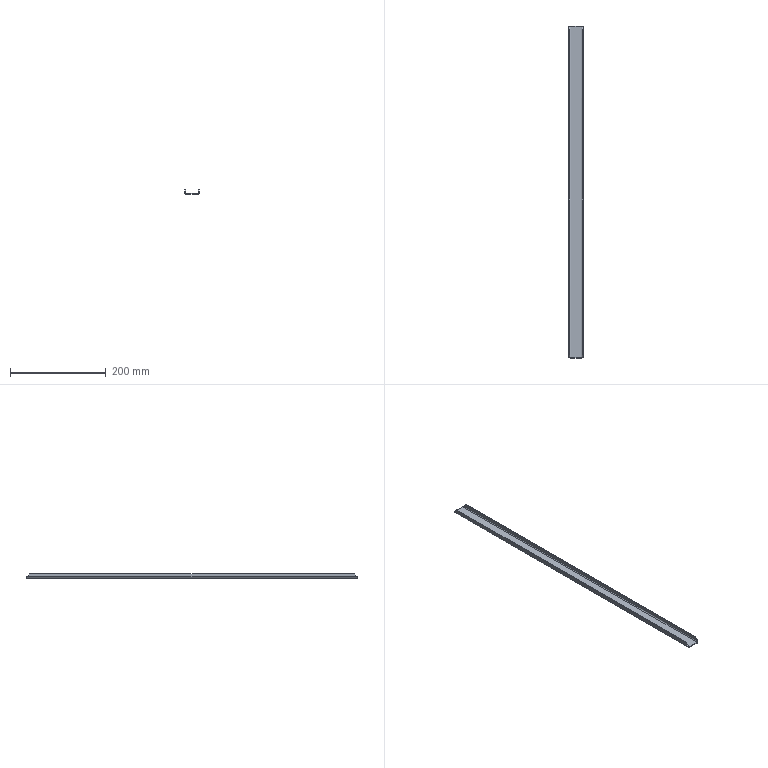Part | NX | features solid 2 | 1 solid | 22 faces | box 30 x 694.177 x 10 mm | volume 60022 mm3 | plane 14 | spline 4 | cylinder 4 | commonest cylinder face diameters 4 x2 8 x2
STEP:
#1=CARTESIAN_POINT('',(1379.,-1435.089,1444.8));
#2=VERTEX_POINT('',#1);
#3=CARTESIAN_POINT('',(1401.,-1435.089,1444.8));
#4=VERTEX_POINT('',#3);
#5=CARTESIAN_POINT('',(1405.,-1435.089,1444.8));
#6=DIRECTION('',(1.,0.,0.));
#7=VECTOR('',#6,1000.);
#8=LINE('',#5,#7);
#9=EDGE_CURVE('',#2,#4,#8,.T.);
#10=ORIENTED_EDGE('',*,*,#9,.T.);
#11=CARTESIAN_POINT('',(1401.,-1435.089,1446.8));
#12=VERTEX_POINT('',#11);
#13=CARTESIAN_POINT('',(1401.,-1435.089,1446.8));
#14=DIRECTION('',(0.,0.,1.));
#15=VECTOR('',#14,1000.);
#16=LINE('',#13,#15);
#17=EDGE_CURVE('',#4,#12,#16,.T.);
#18=ORIENTED_EDGE('',*,*,#17,.T.);
#19=CARTESIAN_POINT('',(1379.,-1435.089,1446.8));
#20=VERTEX_POINT('',#19);
#21=CARTESIAN_POINT('',(1405.,-1435.089,1446.8));
#22=DIRECTION('',(1.,0.,0.));
#23=VECTOR('',#22,1000.);
#24=LINE('',#21,#23);
#25=EDGE_CURVE('',#20,#12,#24,.T.);
#26=ORIENTED_EDGE('',*,*,#25,.F.);
#27=CARTESIAN_POINT('',(1379.,-1435.089,1446.8));
#28=DIRECTION('',(0.,0.,1.));
#29=VECTOR('',#28,1000.);
#30=LINE('',#27,#29);
#31=EDGE_CURVE('',#2,#20,#30,.T.);
#32=ORIENTED_EDGE('',*,*,#31,.F.);
#33=EDGE_LOOP('',(#10,#18,#26,#32));
#34=FACE_BOUND('',#33,.T.);
#35=CARTESIAN_POINT('',(1405.,-1435.089,1446.8));
#36=DIRECTION('',(0.,1.,0.));
#37=DIRECTION('',(0.,0.,-1.));
#38=AXIS2_PLACEMENT_3D('',#35,#36,#37);
#39=PLANE('',#38);
#40=ADVANCED_FACE('',(#34),#39,.F.);
#41=CARTESIAN_POINT('',(1403.,-1433.089,1448.8));
#42=VERTEX_POINT('',#41);
#43=CARTESIAN_POINT('',(1405.,-1433.089,1448.8));
#44=VERTEX_POINT('',#43);
#45=CARTESIAN_POINT('',(1405.,-1433.089,1448.8));
#46=DIRECTION('',(1.,0.,0.));
#47=VECTOR('',#46,1000.);
#48=LINE('',#45,#47);
#49=EDGE_CURVE('',#42,#44,#48,.T.);
#50=ORIENTED_EDGE('',*,*,#49,.F.);
#51=CARTESIAN_POINT('',(1401.,-1435.089,1446.8));
#52=CARTESIAN_POINT('',(1402.172,-1435.089,1446.8));
#53=CARTESIAN_POINT('',(1403.,-1434.26,1447.628));
#54=CARTESIAN_POINT('',(1403.,-1433.089,1448.8));
#55=(BOUNDED_CURVE()B_SPLINE_CURVE(3,(#51,#52,#53,#54),.UNSPECIFIED.,.F.,.F.)B_SPLINE_CURVE_WITH_KNOTS((4,4),(3.142,4.712),.PIECEWISE_BEZIER_KNOTS.)CURVE()GEOMETRIC_REPRESENTATION_ITEM()RATIONAL_B_SPLINE_CURVE((1.,0.8047,0.8047,1.))REPRESENTATION_ITEM(''));
#56=EDGE_CURVE('',#12,#42,#55,.T.);
#57=ORIENTED_EDGE('',*,*,#56,.F.);
#58=ORIENTED_EDGE('',*,*,#17,.F.);
#59=CARTESIAN_POINT('',(1401.,-1435.089,1444.8));
#60=CARTESIAN_POINT('',(1403.343,-1435.089,1444.8));
#61=CARTESIAN_POINT('',(1405.,-1434.26,1446.457));
#62=CARTESIAN_POINT('',(1405.,-1433.089,1448.8));
#63=(BOUNDED_CURVE()B_SPLINE_CURVE(3,(#59,#60,#61,#62),.UNSPECIFIED.,.F.,.F.)B_SPLINE_CURVE_WITH_KNOTS((4,4),(3.142,4.712),.PIECEWISE_BEZIER_KNOTS.)CURVE()GEOMETRIC_REPRESENTATION_ITEM()RATIONAL_B_SPLINE_CURVE((1.,0.8047,0.8047,1.))REPRESENTATION_ITEM(''));
#64=EDGE_CURVE('',#4,#44,#63,.T.);
#65=ORIENTED_EDGE('',*,*,#64,.T.);
#66=EDGE_LOOP('',(#50,#57,#58,#65));
#67=FACE_BOUND('',#66,.T.);
#68=CARTESIAN_POINT('',(1401.,-1435.089,1444.8));
#69=CARTESIAN_POINT('',(1401.,-1435.089,1445.467));
#70=CARTESIAN_POINT('',(1401.,-1435.089,1446.133));
#71=CARTESIAN_POINT('',(1401.,-1435.089,1446.8));
#72=CARTESIAN_POINT('',(1403.,-1435.089,1444.8));
#73=CARTESIAN_POINT('',(1402.667,-1435.089,1445.467));
#74=CARTESIAN_POINT('',(1402.333,-1435.089,1446.133));
#75=CARTESIAN_POINT('',(1402.,-1435.089,1446.8));
#76=CARTESIAN_POINT('',(1405.,-1434.422,1446.133));
#77=CARTESIAN_POINT('',(1404.333,-1434.422,1446.578));
#78=CARTESIAN_POINT('',(1403.667,-1434.422,1447.022));
#79=CARTESIAN_POINT('',(1403.,-1434.422,1447.467));
#80=CARTESIAN_POINT('',(1405.,-1433.089,1448.8));
#81=CARTESIAN_POINT('',(1404.333,-1433.089,1448.8));
#82=CARTESIAN_POINT('',(1403.667,-1433.089,1448.8));
#83=CARTESIAN_POINT('',(1403.,-1433.089,1448.8));
#84=(BOUNDED_SURFACE()B_SPLINE_SURFACE(3,3,((#68,#69,#70,#71),(#72,#73,#74,#75),(#76,#77,#78,#79),(#80,#81,#82,#83)),.UNSPECIFIED.,.F.,.F.,.F.)B_SPLINE_SURFACE_WITH_KNOTS((4,4),(4,4),(0.5,0.75),(0.,1.),.PIECEWISE_BEZIER_KNOTS.)GEOMETRIC_REPRESENTATION_ITEM()RATIONAL_B_SPLINE_SURFACE(((1.,1.,1.,1.),(0.6667,0.6667,0.6667,0.6667),(0.5,0.5,0.5,0.5),(0.5,0.5,0.5,0.5)))REPRESENTATION_ITEM('')SURFACE());
#85=ADVANCED_FACE('',(#67),#84,.T.);
#86=CARTESIAN_POINT('',(1375.,-1433.089,1448.8));
#87=VERTEX_POINT('',#86);
#88=CARTESIAN_POINT('',(1377.,-1433.089,1448.8));
#89=VERTEX_POINT('',#88);
#90=CARTESIAN_POINT('',(1377.,-1433.089,1448.8));
#91=DIRECTION('',(1.,0.,0.));
#92=VECTOR('',#91,1000.);
#93=LINE('',#90,#92);
#94=EDGE_CURVE('',#87,#89,#93,.T.);
#95=ORIENTED_EDGE('',*,*,#94,.T.);
#96=CARTESIAN_POINT('',(1377.,-1427.089,1454.8));
#97=VERTEX_POINT('',#96);
#98=CARTESIAN_POINT('',(1377.,-1436.294,1445.594));
#99=DIRECTION('',(0.,-0.7071,-0.7071));
#100=VECTOR('',#99,1000.);
#101=LINE('',#98,#100);
#102=EDGE_CURVE('',#97,#89,#101,.T.);
#103=ORIENTED_EDGE('',*,*,#102,.F.);
#104=CARTESIAN_POINT('',(1375.,-1427.089,1454.8));
#105=VERTEX_POINT('',#104);
#106=CARTESIAN_POINT('',(1377.,-1427.089,1454.8));
#107=DIRECTION('',(1.,0.,0.));
#108=VECTOR('',#107,1000.);
#109=LINE('',#106,#108);
#110=EDGE_CURVE('',#105,#97,#109,.T.);
#111=ORIENTED_EDGE('',*,*,#110,.F.);
#112=CARTESIAN_POINT('',(1375.,-1436.294,1445.594));
#113=DIRECTION('',(0.,-0.7071,-0.7071));
#114=VECTOR('',#113,1000.);
#115=LINE('',#112,#114);
#116=EDGE_CURVE('',#105,#87,#115,.T.);
#117=ORIENTED_EDGE('',*,*,#116,.T.);
#118=EDGE_LOOP('',(#95,#103,#111,#117));
#119=FACE_BOUND('',#118,.T.);
#120=CARTESIAN_POINT('',(1377.,-1436.294,1445.594));
#121=DIRECTION('',(0.,0.7071,-0.7071));
#122=DIRECTION('',(-1.,0.,0.));
#123=AXIS2_PLACEMENT_3D('',#120,#121,#122);
#124=PLANE('',#123);
#125=ADVANCED_FACE('',(#119),#124,.F.);
#126=ORIENTED_EDGE('',*,*,#31,.T.);
#127=CARTESIAN_POINT('',(1377.,-1433.089,1448.8));
#128=CARTESIAN_POINT('',(1377.,-1434.26,1447.628));
#129=CARTESIAN_POINT('',(1377.828,-1435.089,1446.8));
#130=CARTESIAN_POINT('',(1379.,-1435.089,1446.8));
#131=(BOUNDED_CURVE()B_SPLINE_CURVE(3,(#127,#128,#129,#130),.UNSPECIFIED.,.F.,.F.)B_SPLINE_CURVE_WITH_KNOTS((4,4),(1.571,3.142),.PIECEWISE_BEZIER_KNOTS.)CURVE()GEOMETRIC_REPRESENTATION_ITEM()RATIONAL_B_SPLINE_CURVE((1.,0.8047,0.8047,1.))REPRESENTATION_ITEM(''));
#132=EDGE_CURVE('',#89,#20,#131,.T.);
#133=ORIENTED_EDGE('',*,*,#132,.F.);
#134=ORIENTED_EDGE('',*,*,#94,.F.);
#135=CARTESIAN_POINT('',(1375.,-1433.089,1448.8));
#136=CARTESIAN_POINT('',(1375.,-1434.26,1446.457));
#137=CARTESIAN_POINT('',(1376.657,-1435.089,1444.8));
#138=CARTESIAN_POINT('',(1379.,-1435.089,1444.8));
#139=(BOUNDED_CURVE()B_SPLINE_CURVE(3,(#135,#136,#137,#138),.UNSPECIFIED.,.F.,.F.)B_SPLINE_CURVE_WITH_KNOTS((4,4),(1.571,3.142),.PIECEWISE_BEZIER_KNOTS.)CURVE()GEOMETRIC_REPRESENTATION_ITEM()RATIONAL_B_SPLINE_CURVE((1.,0.8047,0.8047,1.))REPRESENTATION_ITEM(''));
#140=EDGE_CURVE('',#87,#2,#139,.T.);
#141=ORIENTED_EDGE('',*,*,#140,.T.);
#142=EDGE_LOOP('',(#126,#133,#134,#141));
#143=FACE_BOUND('',#142,.T.);
#144=CARTESIAN_POINT('',(1375.,-1433.089,1448.8));
#145=CARTESIAN_POINT('',(1375.667,-1433.089,1448.8));
#146=CARTESIAN_POINT('',(1376.333,-1433.089,1448.8));
#147=CARTESIAN_POINT('',(1377.,-1433.089,1448.8));
#148=CARTESIAN_POINT('',(1375.,-1434.422,1446.133));
#149=CARTESIAN_POINT('',(1375.667,-1434.422,1446.578));
#150=CARTESIAN_POINT('',(1376.333,-1434.422,1447.022));
#151=CARTESIAN_POINT('',(1377.,-1434.422,1447.467));
#152=CARTESIAN_POINT('',(1377.,-1435.089,1444.8));
#153=CARTESIAN_POINT('',(1377.333,-1435.089,1445.467));
#154=CARTESIAN_POINT('',(1377.667,-1435.089,1446.133));
#155=CARTESIAN_POINT('',(1378.,-1435.089,1446.8));
#156=CARTESIAN_POINT('',(1379.,-1435.089,1444.8));
#157=CARTESIAN_POINT('',(1379.,-1435.089,1445.467));
#158=CARTESIAN_POINT('',(1379.,-1435.089,1446.133));
#159=CARTESIAN_POINT('',(1379.,-1435.089,1446.8));
#160=(BOUNDED_SURFACE()B_SPLINE_SURFACE(3,3,((#144,#145,#146,#147),(#148,#149,#150,#151),(#152,#153,#154,#155),(#156,#157,#158,#159)),.UNSPECIFIED.,.F.,.F.,.F.)B_SPLINE_SURFACE_WITH_KNOTS((4,4),(4,4),(0.25,0.5),(0.,1.),.PIECEWISE_BEZIER_KNOTS.)GEOMETRIC_REPRESENTATION_ITEM()RATIONAL_B_SPLINE_SURFACE(((0.5,0.5,0.5,0.5),(0.5,0.5,0.5,0.5),(0.6667,0.6667,0.6667,0.6667),(1.,1.,1.,1.)))REPRESENTATION_ITEM('')SURFACE());
#161=ADVANCED_FACE('',(#143),#160,.T.);
#162=ORIENTED_EDGE('',*,*,#49,.T.);
#163=CARTESIAN_POINT('',(1405.,-1427.089,1454.8));
#164=VERTEX_POINT('',#163);
#165=CARTESIAN_POINT('',(1405.,-1431.294,1450.594));
#166=DIRECTION('',(0.,0.7071,0.7071));
#167=VECTOR('',#166,1000.);
#168=LINE('',#165,#167);
#169=EDGE_CURVE('',#44,#164,#168,.T.);
#170=ORIENTED_EDGE('',*,*,#169,.T.);
#171=CARTESIAN_POINT('',(1403.,-1427.089,1454.8));
#172=VERTEX_POINT('',#171);
#173=CARTESIAN_POINT('',(1405.,-1427.089,1454.8));
#174=DIRECTION('',(1.,0.,0.));
#175=VECTOR('',#174,1000.);
#176=LINE('',#173,#175);
#177=EDGE_CURVE('',#172,#164,#176,.T.);
#178=ORIENTED_EDGE('',*,*,#177,.F.);
#179=CARTESIAN_POINT('',(1403.,-1431.294,1450.594));
#180=DIRECTION('',(0.,0.7071,0.7071));
#181=VECTOR('',#180,1000.);
#182=LINE('',#179,#181);
#183=EDGE_CURVE('',#42,#172,#182,.T.);
#184=ORIENTED_EDGE('',*,*,#183,.F.);
#185=EDGE_LOOP('',(#162,#170,#178,#184));
#186=FACE_BOUND('',#185,.T.);
#187=CARTESIAN_POINT('',(1405.,-1431.294,1450.594));
#188=DIRECTION('',(0.,0.7071,-0.7071));
#189=DIRECTION('',(-1.,0.,0.));
#190=AXIS2_PLACEMENT_3D('',#187,#188,#189);
#191=PLANE('',#190);
#192=ADVANCED_FACE('',(#186),#191,.F.);
#193=CARTESIAN_POINT('',(1401.,-740.911,1444.8));
#194=VERTEX_POINT('',#193);
#195=CARTESIAN_POINT('',(1379.,-740.911,1444.8));
#196=VERTEX_POINT('',#195);
#197=CARTESIAN_POINT('',(1405.,-740.911,1444.8));
#198=DIRECTION('',(-1.,0.,0.));
#199=VECTOR('',#198,1000.);
#200=LINE('',#197,#199);
#201=EDGE_CURVE('',#194,#196,#200,.T.);
#202=ORIENTED_EDGE('',*,*,#201,.T.);
#203=CARTESIAN_POINT('',(1379.,-740.911,1446.8));
#204=VERTEX_POINT('',#203);
#205=CARTESIAN_POINT('',(1379.,-740.911,1446.8));
#206=DIRECTION('',(0.,0.,1.));
#207=VECTOR('',#206,1000.);
#208=LINE('',#205,#207);
#209=EDGE_CURVE('',#196,#204,#208,.T.);
#210=ORIENTED_EDGE('',*,*,#209,.T.);
#211=CARTESIAN_POINT('',(1401.,-740.911,1446.8));
#212=VERTEX_POINT('',#211);
#213=CARTESIAN_POINT('',(1405.,-740.911,1446.8));
#214=DIRECTION('',(-1.,0.,0.));
#215=VECTOR('',#214,1000.);
#216=LINE('',#213,#215);
#217=EDGE_CURVE('',#212,#204,#216,.T.);
#218=ORIENTED_EDGE('',*,*,#217,.F.);
#219=CARTESIAN_POINT('',(1401.,-740.911,1446.8));
#220=DIRECTION('',(0.,0.,1.));
#221=VECTOR('',#220,1000.);
#222=LINE('',#219,#221);
#223=EDGE_CURVE('',#194,#212,#222,.T.);
#224=ORIENTED_EDGE('',*,*,#223,.F.);
#225=EDGE_LOOP('',(#202,#210,#218,#224));
#226=FACE_BOUND('',#225,.T.);
#227=CARTESIAN_POINT('',(1405.,-740.911,1446.8));
#228=DIRECTION('',(0.,-1.,0.));
#229=DIRECTION('',(-1.,0.,0.));
#230=AXIS2_PLACEMENT_3D('',#227,#228,#229);
#231=PLANE('',#230);
#232=ADVANCED_FACE('',(#226),#231,.F.);
#233=CARTESIAN_POINT('',(1375.,-742.911,1448.8));
#234=VERTEX_POINT('',#233);
#235=CARTESIAN_POINT('',(1377.,-742.911,1448.8));
#236=VERTEX_POINT('',#235);
#237=CARTESIAN_POINT('',(1377.,-742.911,1448.8));
#238=DIRECTION('',(1.,0.,0.));
#239=VECTOR('',#238,1000.);
#240=LINE('',#237,#239);
#241=EDGE_CURVE('',#234,#236,#240,.T.);
#242=ORIENTED_EDGE('',*,*,#241,.T.);
#243=CARTESIAN_POINT('',(1379.,-740.911,1446.8));
#244=CARTESIAN_POINT('',(1377.828,-740.911,1446.8));
#245=CARTESIAN_POINT('',(1377.,-741.74,1447.628));
#246=CARTESIAN_POINT('',(1377.,-742.911,1448.8));
#247=(BOUNDED_CURVE()B_SPLINE_CURVE(3,(#243,#244,#245,#246),.UNSPECIFIED.,.F.,.F.)B_SPLINE_CURVE_WITH_KNOTS((4,4),(0.,1.571),.PIECEWISE_BEZIER_KNOTS.)CURVE()GEOMETRIC_REPRESENTATION_ITEM()RATIONAL_B_SPLINE_CURVE((1.,0.8047,0.8047,1.))REPRESENTATION_ITEM(''));
#248=EDGE_CURVE('',#204,#236,#247,.T.);
#249=ORIENTED_EDGE('',*,*,#248,.F.);
#250=ORIENTED_EDGE('',*,*,#209,.F.);
#251=CARTESIAN_POINT('',(1379.,-740.911,1444.8));
#252=CARTESIAN_POINT('',(1376.657,-740.911,1444.8));
#253=CARTESIAN_POINT('',(1375.,-741.74,1446.457));
#254=CARTESIAN_POINT('',(1375.,-742.911,1448.8));
#255=(BOUNDED_CURVE()B_SPLINE_CURVE(3,(#251,#252,#253,#254),.UNSPECIFIED.,.F.,.F.)B_SPLINE_CURVE_WITH_KNOTS((4,4),(0.,1.571),.PIECEWISE_BEZIER_KNOTS.)CURVE()GEOMETRIC_REPRESENTATION_ITEM()RATIONAL_B_SPLINE_CURVE((1.,0.8047,0.8047,1.))REPRESENTATION_ITEM(''));
#256=EDGE_CURVE('',#196,#234,#255,.T.);
#257=ORIENTED_EDGE('',*,*,#256,.T.);
#258=EDGE_LOOP('',(#242,#249,#250,#257));
#259=FACE_BOUND('',#258,.T.);
#260=CARTESIAN_POINT('',(1379.,-740.911,1444.8));
#261=CARTESIAN_POINT('',(1379.,-740.911,1445.467));
#262=CARTESIAN_POINT('',(1379.,-740.911,1446.133));
#263=CARTESIAN_POINT('',(1379.,-740.911,1446.8));
#264=CARTESIAN_POINT('',(1377.,-740.911,1444.8));
#265=CARTESIAN_POINT('',(1377.333,-740.911,1445.467));
#266=CARTESIAN_POINT('',(1377.667,-740.911,1446.133));
#267=CARTESIAN_POINT('',(1378.,-740.911,1446.8));
#268=CARTESIAN_POINT('',(1375.,-741.578,1446.133));
#269=CARTESIAN_POINT('',(1375.667,-741.578,1446.578));
#270=CARTESIAN_POINT('',(1376.333,-741.578,1447.022));
#271=CARTESIAN_POINT('',(1377.,-741.578,1447.467));
#272=CARTESIAN_POINT('',(1375.,-742.911,1448.8));
#273=CARTESIAN_POINT('',(1375.667,-742.911,1448.8));
#274=CARTESIAN_POINT('',(1376.333,-742.911,1448.8));
#275=CARTESIAN_POINT('',(1377.,-742.911,1448.8));
#276=(BOUNDED_SURFACE()B_SPLINE_SURFACE(3,3,((#260,#261,#262,#263),(#264,#265,#266,#267),(#268,#269,#270,#271),(#272,#273,#274,#275)),.UNSPECIFIED.,.F.,.F.,.F.)B_SPLINE_SURFACE_WITH_KNOTS((4,4),(4,4),(0.,0.25),(0.,1.),.PIECEWISE_BEZIER_KNOTS.)GEOMETRIC_REPRESENTATION_ITEM()RATIONAL_B_SPLINE_SURFACE(((1.,1.,1.,1.),(0.6667,0.6667,0.6667,0.6667),(0.5,0.5,0.5,0.5),(0.5,0.5,0.5,0.5)))REPRESENTATION_ITEM('')SURFACE());
#277=ADVANCED_FACE('',(#259),#276,.T.);
#278=CARTESIAN_POINT('',(1375.,-748.911,1454.8));
#279=VERTEX_POINT('',#278);
#280=CARTESIAN_POINT('',(1377.,-748.911,1454.8));
#281=VERTEX_POINT('',#280);
#282=CARTESIAN_POINT('',(1377.,-748.911,1454.8));
#283=DIRECTION('',(1.,0.,0.));
#284=VECTOR('',#283,1000.);
#285=LINE('',#282,#284);
#286=EDGE_CURVE('',#279,#281,#285,.T.);
#287=ORIENTED_EDGE('',*,*,#286,.T.);
#288=CARTESIAN_POINT('',(1377.,-1087.206,1793.094));
#289=DIRECTION('',(0.,-0.7071,0.7071));
#290=VECTOR('',#289,1000.);
#291=LINE('',#288,#290);
#292=EDGE_CURVE('',#236,#281,#291,.T.);
#293=ORIENTED_EDGE('',*,*,#292,.F.);
#294=ORIENTED_EDGE('',*,*,#241,.F.);
#295=CARTESIAN_POINT('',(1375.,-1087.206,1793.094));
#296=DIRECTION('',(0.,-0.7071,0.7071));
#297=VECTOR('',#296,1000.);
#298=LINE('',#295,#297);
#299=EDGE_CURVE('',#234,#279,#298,.T.);
#300=ORIENTED_EDGE('',*,*,#299,.T.);
#301=EDGE_LOOP('',(#287,#293,#294,#300));
#302=FACE_BOUND('',#301,.T.);
#303=CARTESIAN_POINT('',(1377.,-1087.206,1793.094));
#304=DIRECTION('',(0.,-0.7071,-0.7071));
#305=DIRECTION('',(0.,0.7071,-0.7071));
#306=AXIS2_PLACEMENT_3D('',#303,#304,#305);
#307=PLANE('',#306);
#308=ADVANCED_FACE('',(#302),#307,.F.);
#309=ORIENTED_EDGE('',*,*,#223,.T.);
#310=CARTESIAN_POINT('',(1403.,-742.911,1448.8));
#311=VERTEX_POINT('',#310);
#312=CARTESIAN_POINT('',(1403.,-742.911,1448.8));
#313=CARTESIAN_POINT('',(1403.,-741.74,1447.628));
#314=CARTESIAN_POINT('',(1402.172,-740.911,1446.8));
#315=CARTESIAN_POINT('',(1401.,-740.911,1446.8));
#316=(BOUNDED_CURVE()B_SPLINE_CURVE(3,(#312,#313,#314,#315),.UNSPECIFIED.,.F.,.F.)B_SPLINE_CURVE_WITH_KNOTS((4,4),(4.712,6.283),.PIECEWISE_BEZIER_KNOTS.)CURVE()GEOMETRIC_REPRESENTATION_ITEM()RATIONAL_B_SPLINE_CURVE((1.,0.8047,0.8047,1.))REPRESENTATION_ITEM(''));
#317=EDGE_CURVE('',#311,#212,#316,.T.);
#318=ORIENTED_EDGE('',*,*,#317,.F.);
#319=CARTESIAN_POINT('',(1405.,-742.911,1448.8));
#320=VERTEX_POINT('',#319);
#321=CARTESIAN_POINT('',(1405.,-742.911,1448.8));
#322=DIRECTION('',(1.,0.,0.));
#323=VECTOR('',#322,1000.);
#324=LINE('',#321,#323);
#325=EDGE_CURVE('',#311,#320,#324,.T.);
#326=ORIENTED_EDGE('',*,*,#325,.T.);
#327=CARTESIAN_POINT('',(1405.,-742.911,1448.8));
#328=CARTESIAN_POINT('',(1405.,-741.74,1446.457));
#329=CARTESIAN_POINT('',(1403.343,-740.911,1444.8));
#330=CARTESIAN_POINT('',(1401.,-740.911,1444.8));
#331=(BOUNDED_CURVE()B_SPLINE_CURVE(3,(#327,#328,#329,#330),.UNSPECIFIED.,.F.,.F.)B_SPLINE_CURVE_WITH_KNOTS((4,4),(4.712,6.283),.PIECEWISE_BEZIER_KNOTS.)CURVE()GEOMETRIC_REPRESENTATION_ITEM()RATIONAL_B_SPLINE_CURVE((1.,0.8047,0.8047,1.))REPRESENTATION_ITEM(''));
#332=EDGE_CURVE('',#320,#194,#331,.T.);
#333=ORIENTED_EDGE('',*,*,#332,.T.);
#334=EDGE_LOOP('',(#309,#318,#326,#333));
#335=FACE_BOUND('',#334,.T.);
#336=CARTESIAN_POINT('',(1405.,-742.911,1448.8));
#337=CARTESIAN_POINT('',(1404.333,-742.911,1448.8));
#338=CARTESIAN_POINT('',(1403.667,-742.911,1448.8));
#339=CARTESIAN_POINT('',(1403.,-742.911,1448.8));
#340=CARTESIAN_POINT('',(1405.,-741.578,1446.133));
#341=CARTESIAN_POINT('',(1404.333,-741.578,1446.578));
#342=CARTESIAN_POINT('',(1403.667,-741.578,1447.022));
#343=CARTESIAN_POINT('',(1403.,-741.578,1447.467));
#344=CARTESIAN_POINT('',(1403.,-740.911,1444.8));
#345=CARTESIAN_POINT('',(1402.667,-740.911,1445.467));
#346=CARTESIAN_POINT('',(1402.333,-740.911,1446.133));
#347=CARTESIAN_POINT('',(1402.,-740.911,1446.8));
#348=CARTESIAN_POINT('',(1401.,-740.911,1444.8));
#349=CARTESIAN_POINT('',(1401.,-740.911,1445.467));
#350=CARTESIAN_POINT('',(1401.,-740.911,1446.133));
#351=CARTESIAN_POINT('',(1401.,-740.911,1446.8));
#352=(BOUNDED_SURFACE()B_SPLINE_SURFACE(3,3,((#336,#337,#338,#339),(#340,#341,#342,#343),(#344,#345,#346,#347),(#348,#349,#350,#351)),.UNSPECIFIED.,.F.,.F.,.F.)B_SPLINE_SURFACE_WITH_KNOTS((4,4),(4,4),(0.75,1.),(0.,1.),.PIECEWISE_BEZIER_KNOTS.)GEOMETRIC_REPRESENTATION_ITEM()RATIONAL_B_SPLINE_SURFACE(((0.5,0.5,0.5,0.5),(0.5,0.5,0.5,0.5),(0.6667,0.6667,0.6667,0.6667),(1.,1.,1.,1.)))REPRESENTATION_ITEM('')SURFACE());
#353=ADVANCED_FACE('',(#335),#352,.T.);
#354=CARTESIAN_POINT('',(1403.,-748.911,1454.8));
#355=VERTEX_POINT('',#354);
#356=CARTESIAN_POINT('',(1403.,-1092.206,1798.094));
#357=DIRECTION('',(0.,0.7071,-0.7071));
#358=VECTOR('',#357,1000.);
#359=LINE('',#356,#358);
#360=EDGE_CURVE('',#355,#311,#359,.T.);
#361=ORIENTED_EDGE('',*,*,#360,.F.);
#362=CARTESIAN_POINT('',(1405.,-748.911,1454.8));
#363=VERTEX_POINT('',#362);
#364=CARTESIAN_POINT('',(1405.,-748.911,1454.8));
#365=DIRECTION('',(1.,0.,0.));
#366=VECTOR('',#365,1000.);
#367=LINE('',#364,#366);
#368=EDGE_CURVE('',#355,#363,#367,.T.);
#369=ORIENTED_EDGE('',*,*,#368,.T.);
#370=CARTESIAN_POINT('',(1405.,-1092.206,1798.094));
#371=DIRECTION('',(0.,0.7071,-0.7071));
#372=VECTOR('',#371,1000.);
#373=LINE('',#370,#372);
#374=EDGE_CURVE('',#363,#320,#373,.T.);
#375=ORIENTED_EDGE('',*,*,#374,.T.);
#376=ORIENTED_EDGE('',*,*,#325,.F.);
#377=EDGE_LOOP('',(#361,#369,#375,#376));
#378=FACE_BOUND('',#377,.T.);
#379=CARTESIAN_POINT('',(1405.,-1092.206,1798.094));
#380=DIRECTION('',(0.,-0.7071,-0.7071));
#381=DIRECTION('',(0.,0.7071,-0.7071));
#382=AXIS2_PLACEMENT_3D('',#379,#380,#381);
#383=PLANE('',#382);
#384=ADVANCED_FACE('',(#378),#383,.F.);
#385=CARTESIAN_POINT('',(1377.,-1435.5,1454.8));
#386=DIRECTION('',(0.,1.,0.));
#387=VECTOR('',#386,1000.);
#388=LINE('',#385,#387);
#389=EDGE_CURVE('',#97,#281,#388,.T.);
#390=ORIENTED_EDGE('',*,*,#389,.F.);
#391=ORIENTED_EDGE('',*,*,#102,.T.);
#392=CARTESIAN_POINT('',(1377.,-1435.5,1448.8));
#393=DIRECTION('',(0.,1.,0.));
#394=VECTOR('',#393,1000.);
#395=LINE('',#392,#394);
#396=EDGE_CURVE('',#89,#236,#395,.T.);
#397=ORIENTED_EDGE('',*,*,#396,.T.);
#398=ORIENTED_EDGE('',*,*,#292,.T.);
#399=EDGE_LOOP('',(#390,#391,#397,#398));
#400=FACE_BOUND('',#399,.T.);
#401=CARTESIAN_POINT('',(1377.,-1435.5,1444.8));
#402=DIRECTION('',(-1.,0.,0.));
#403=DIRECTION('',(0.,0.,1.));
#404=AXIS2_PLACEMENT_3D('',#401,#402,#403);
#405=PLANE('',#404);
#406=ADVANCED_FACE('',(#400),#405,.F.);
#407=ORIENTED_EDGE('',*,*,#396,.F.);
#408=ORIENTED_EDGE('',*,*,#132,.T.);
#409=CARTESIAN_POINT('',(1379.,-1435.5,1446.8));
#410=DIRECTION('',(0.,1.,0.));
#411=VECTOR('',#410,1000.);
#412=LINE('',#409,#411);
#413=EDGE_CURVE('',#20,#204,#412,.T.);
#414=ORIENTED_EDGE('',*,*,#413,.T.);
#415=ORIENTED_EDGE('',*,*,#248,.T.);
#416=EDGE_LOOP('',(#407,#408,#414,#415));
#417=FACE_BOUND('',#416,.T.);
#418=CARTESIAN_POINT('',(1379.,-1435.5,1448.8));
#419=DIRECTION('',(0.,1.,0.));
#420=DIRECTION('',(0.,0.,-1.));
#421=AXIS2_PLACEMENT_3D('',#418,#419,#420);
#422=CYLINDRICAL_SURFACE('',#421,2.);
#423=ADVANCED_FACE('',(#417),#422,.F.);
#424=ORIENTED_EDGE('',*,*,#413,.F.);
#425=ORIENTED_EDGE('',*,*,#25,.T.);
#426=CARTESIAN_POINT('',(1401.,-1435.5,1446.8));
#427=DIRECTION('',(0.,1.,0.));
#428=VECTOR('',#427,1000.);
#429=LINE('',#426,#428);
#430=EDGE_CURVE('',#12,#212,#429,.T.);
#431=ORIENTED_EDGE('',*,*,#430,.T.);
#432=ORIENTED_EDGE('',*,*,#217,.T.);
#433=EDGE_LOOP('',(#424,#425,#431,#432));
#434=FACE_BOUND('',#433,.T.);
#435=CARTESIAN_POINT('',(1405.,-1435.5,1446.8));
#436=DIRECTION('',(0.,0.,-1.));
#437=DIRECTION('',(0.,-1.,0.));
#438=AXIS2_PLACEMENT_3D('',#435,#436,#437);
#439=PLANE('',#438);
#440=ADVANCED_FACE('',(#434),#439,.F.);
#441=ORIENTED_EDGE('',*,*,#430,.F.);
#442=ORIENTED_EDGE('',*,*,#56,.T.);
#443=CARTESIAN_POINT('',(1403.,-1435.5,1448.8));
#444=DIRECTION('',(0.,1.,0.));
#445=VECTOR('',#444,1000.);
#446=LINE('',#443,#445);
#447=EDGE_CURVE('',#42,#311,#446,.T.);
#448=ORIENTED_EDGE('',*,*,#447,.T.);
#449=ORIENTED_EDGE('',*,*,#317,.T.);
#450=EDGE_LOOP('',(#441,#442,#448,#449));
#451=FACE_BOUND('',#450,.T.);
#452=CARTESIAN_POINT('',(1401.,-1435.5,1448.8));
#453=DIRECTION('',(0.,1.,0.));
#454=DIRECTION('',(0.,0.,-1.));
#455=AXIS2_PLACEMENT_3D('',#452,#453,#454);
#456=CYLINDRICAL_SURFACE('',#455,2.);
#457=ADVANCED_FACE('',(#451),#456,.F.);
#458=ORIENTED_EDGE('',*,*,#447,.F.);
#459=ORIENTED_EDGE('',*,*,#183,.T.);
#460=CARTESIAN_POINT('',(1403.,-1435.5,1454.8));
#461=DIRECTION('',(0.,1.,0.));
#462=VECTOR('',#461,1000.);
#463=LINE('',#460,#462);
#464=EDGE_CURVE('',#172,#355,#463,.T.);
#465=ORIENTED_EDGE('',*,*,#464,.T.);
#466=ORIENTED_EDGE('',*,*,#360,.T.);
#467=EDGE_LOOP('',(#458,#459,#465,#466));
#468=FACE_BOUND('',#467,.T.);
#469=CARTESIAN_POINT('',(1403.,-1435.5,1454.8));
#470=DIRECTION('',(1.,0.,0.));
#471=DIRECTION('',(0.,0.,1.));
#472=AXIS2_PLACEMENT_3D('',#469,#470,#471);
#473=PLANE('',#472);
#474=ADVANCED_FACE('',(#468),#473,.F.);
#475=ORIENTED_EDGE('',*,*,#116,.F.);
#476=CARTESIAN_POINT('',(1375.,-1435.5,1454.8));
#477=DIRECTION('',(0.,1.,0.));
#478=VECTOR('',#477,1000.);
#479=LINE('',#476,#478);
#480=EDGE_CURVE('',#105,#279,#479,.T.);
#481=ORIENTED_EDGE('',*,*,#480,.T.);
#482=ORIENTED_EDGE('',*,*,#299,.F.);
#483=CARTESIAN_POINT('',(1375.,-1435.5,1448.8));
#484=DIRECTION('',(0.,1.,0.));
#485=VECTOR('',#484,1000.);
#486=LINE('',#483,#485);
#487=EDGE_CURVE('',#87,#234,#486,.T.);
#488=ORIENTED_EDGE('',*,*,#487,.F.);
#489=EDGE_LOOP('',(#475,#481,#482,#488));
#490=FACE_BOUND('',#489,.T.);
#491=CARTESIAN_POINT('',(1375.,-1435.5,1444.8));
#492=DIRECTION('',(-1.,0.,0.));
#493=DIRECTION('',(0.,0.,1.));
#494=AXIS2_PLACEMENT_3D('',#491,#492,#493);
#495=PLANE('',#494);
#496=ADVANCED_FACE('',(#490),#495,.T.);
#497=ORIENTED_EDGE('',*,*,#140,.F.);
#498=ORIENTED_EDGE('',*,*,#487,.T.);
#499=ORIENTED_EDGE('',*,*,#256,.F.);
#500=CARTESIAN_POINT('',(1379.,-1435.5,1444.8));
#501=DIRECTION('',(0.,1.,0.));
#502=VECTOR('',#501,1000.);
#503=LINE('',#500,#502);
#504=EDGE_CURVE('',#2,#196,#503,.T.);
#505=ORIENTED_EDGE('',*,*,#504,.F.);
#506=EDGE_LOOP('',(#497,#498,#499,#505));
#507=FACE_BOUND('',#506,.T.);
#508=CARTESIAN_POINT('',(1379.,-1435.5,1448.8));
#509=DIRECTION('',(0.,1.,0.));
#510=DIRECTION('',(0.,0.,-1.));
#511=AXIS2_PLACEMENT_3D('',#508,#509,#510);
#512=CYLINDRICAL_SURFACE('',#511,4.);
#513=ADVANCED_FACE('',(#507),#512,.T.);
#514=ORIENTED_EDGE('',*,*,#9,.F.);
#515=ORIENTED_EDGE('',*,*,#504,.T.);
#516=ORIENTED_EDGE('',*,*,#201,.F.);
#517=CARTESIAN_POINT('',(1401.,-1435.5,1444.8));
#518=DIRECTION('',(0.,1.,0.));
#519=VECTOR('',#518,1000.);
#520=LINE('',#517,#519);
#521=EDGE_CURVE('',#4,#194,#520,.T.);
#522=ORIENTED_EDGE('',*,*,#521,.F.);
#523=EDGE_LOOP('',(#514,#515,#516,#522));
#524=FACE_BOUND('',#523,.T.);
#525=CARTESIAN_POINT('',(1405.,-1435.5,1444.8));
#526=DIRECTION('',(0.,0.,-1.));
#527=DIRECTION('',(0.,-1.,0.));
#528=AXIS2_PLACEMENT_3D('',#525,#526,#527);
#529=PLANE('',#528);
#530=ADVANCED_FACE('',(#524),#529,.T.);
#531=ORIENTED_EDGE('',*,*,#64,.F.);
#532=ORIENTED_EDGE('',*,*,#521,.T.);
#533=ORIENTED_EDGE('',*,*,#332,.F.);
#534=CARTESIAN_POINT('',(1405.,-1435.5,1448.8));
#535=DIRECTION('',(0.,1.,0.));
#536=VECTOR('',#535,1000.);
#537=LINE('',#534,#536);
#538=EDGE_CURVE('',#44,#320,#537,.T.);
#539=ORIENTED_EDGE('',*,*,#538,.F.);
#540=EDGE_LOOP('',(#531,#532,#533,#539));
#541=FACE_BOUND('',#540,.T.);
#542=CARTESIAN_POINT('',(1401.,-1435.5,1448.8));
#543=DIRECTION('',(0.,1.,0.));
#544=DIRECTION('',(0.,0.,-1.));
#545=AXIS2_PLACEMENT_3D('',#542,#543,#544);
#546=CYLINDRICAL_SURFACE('',#545,4.);
#547=ADVANCED_FACE('',(#541),#546,.T.);
#548=ORIENTED_EDGE('',*,*,#169,.F.);
#549=ORIENTED_EDGE('',*,*,#538,.T.);
#550=ORIENTED_EDGE('',*,*,#374,.F.);
#551=CARTESIAN_POINT('',(1405.,-1435.5,1454.8));
#552=DIRECTION('',(0.,1.,0.));
#553=VECTOR('',#552,1000.);
#554=LINE('',#551,#553);
#555=EDGE_CURVE('',#164,#363,#554,.T.);
#556=ORIENTED_EDGE('',*,*,#555,.F.);
#557=EDGE_LOOP('',(#548,#549,#550,#556));
#558=FACE_BOUND('',#557,.T.);
#559=CARTESIAN_POINT('',(1405.,-1435.5,1454.8));
#560=DIRECTION('',(1.,0.,0.));
#561=DIRECTION('',(0.,0.,1.));
#562=AXIS2_PLACEMENT_3D('',#559,#560,#561);
#563=PLANE('',#562);
#564=ADVANCED_FACE('',(#558),#563,.T.);
#565=ORIENTED_EDGE('',*,*,#177,.T.);
#566=ORIENTED_EDGE('',*,*,#555,.T.);
#567=ORIENTED_EDGE('',*,*,#368,.F.);
#568=ORIENTED_EDGE('',*,*,#464,.F.);
#569=EDGE_LOOP('',(#565,#566,#567,#568));
#570=FACE_BOUND('',#569,.T.);
#571=CARTESIAN_POINT('',(1405.,-1435.5,1454.8));
#572=DIRECTION('',(0.,0.,-1.));
#573=DIRECTION('',(0.,-1.,0.));
#574=AXIS2_PLACEMENT_3D('',#571,#572,#573);
#575=PLANE('',#574);
#576=ADVANCED_FACE('',(#570),#575,.F.);
#577=ORIENTED_EDGE('',*,*,#110,.T.);
#578=ORIENTED_EDGE('',*,*,#389,.T.);
#579=ORIENTED_EDGE('',*,*,#286,.F.);
#580=ORIENTED_EDGE('',*,*,#480,.F.);
#581=EDGE_LOOP('',(#577,#578,#579,#580));
#582=FACE_BOUND('',#581,.T.);
#583=CARTESIAN_POINT('',(1375.,-1435.5,1454.8));
#584=DIRECTION('',(0.,0.,1.));
#585=DIRECTION('',(1.,0.,0.));
#586=AXIS2_PLACEMENT_3D('',#583,#584,#585);
#587=PLANE('',#586);
#588=ADVANCED_FACE('',(#582),#587,.T.);
#589=CLOSED_SHELL('',(#40,#85,#125,#161,#192,#232,#277,#308,#353,#384,#406,#423,#440,#457,#474,#496,#513,#530,#547,#564,#576,#588));
#590=MANIFOLD_SOLID_BREP('',#589);
#591=(LENGTH_UNIT()NAMED_UNIT(*)SI_UNIT(.MILLI.,.METRE.));
#592=UNCERTAINTY_MEASURE_WITH_UNIT(LENGTH_MEASURE(0.00001),#591,'','');
#593=(NAMED_UNIT(*)PLANE_ANGLE_UNIT()SI_UNIT($,.RADIAN.));
#594=(NAMED_UNIT(*)SI_UNIT($,.STERADIAN.)SOLID_ANGLE_UNIT());
#595=(GEOMETRIC_REPRESENTATION_CONTEXT(3)GLOBAL_UNCERTAINTY_ASSIGNED_CONTEXT((#592))GLOBAL_UNIT_ASSIGNED_CONTEXT((#591,#593,#594))REPRESENTATION_CONTEXT('',''));
#596=ADVANCED_BREP_SHAPE_REPRESENTATION('',(#590),#595);